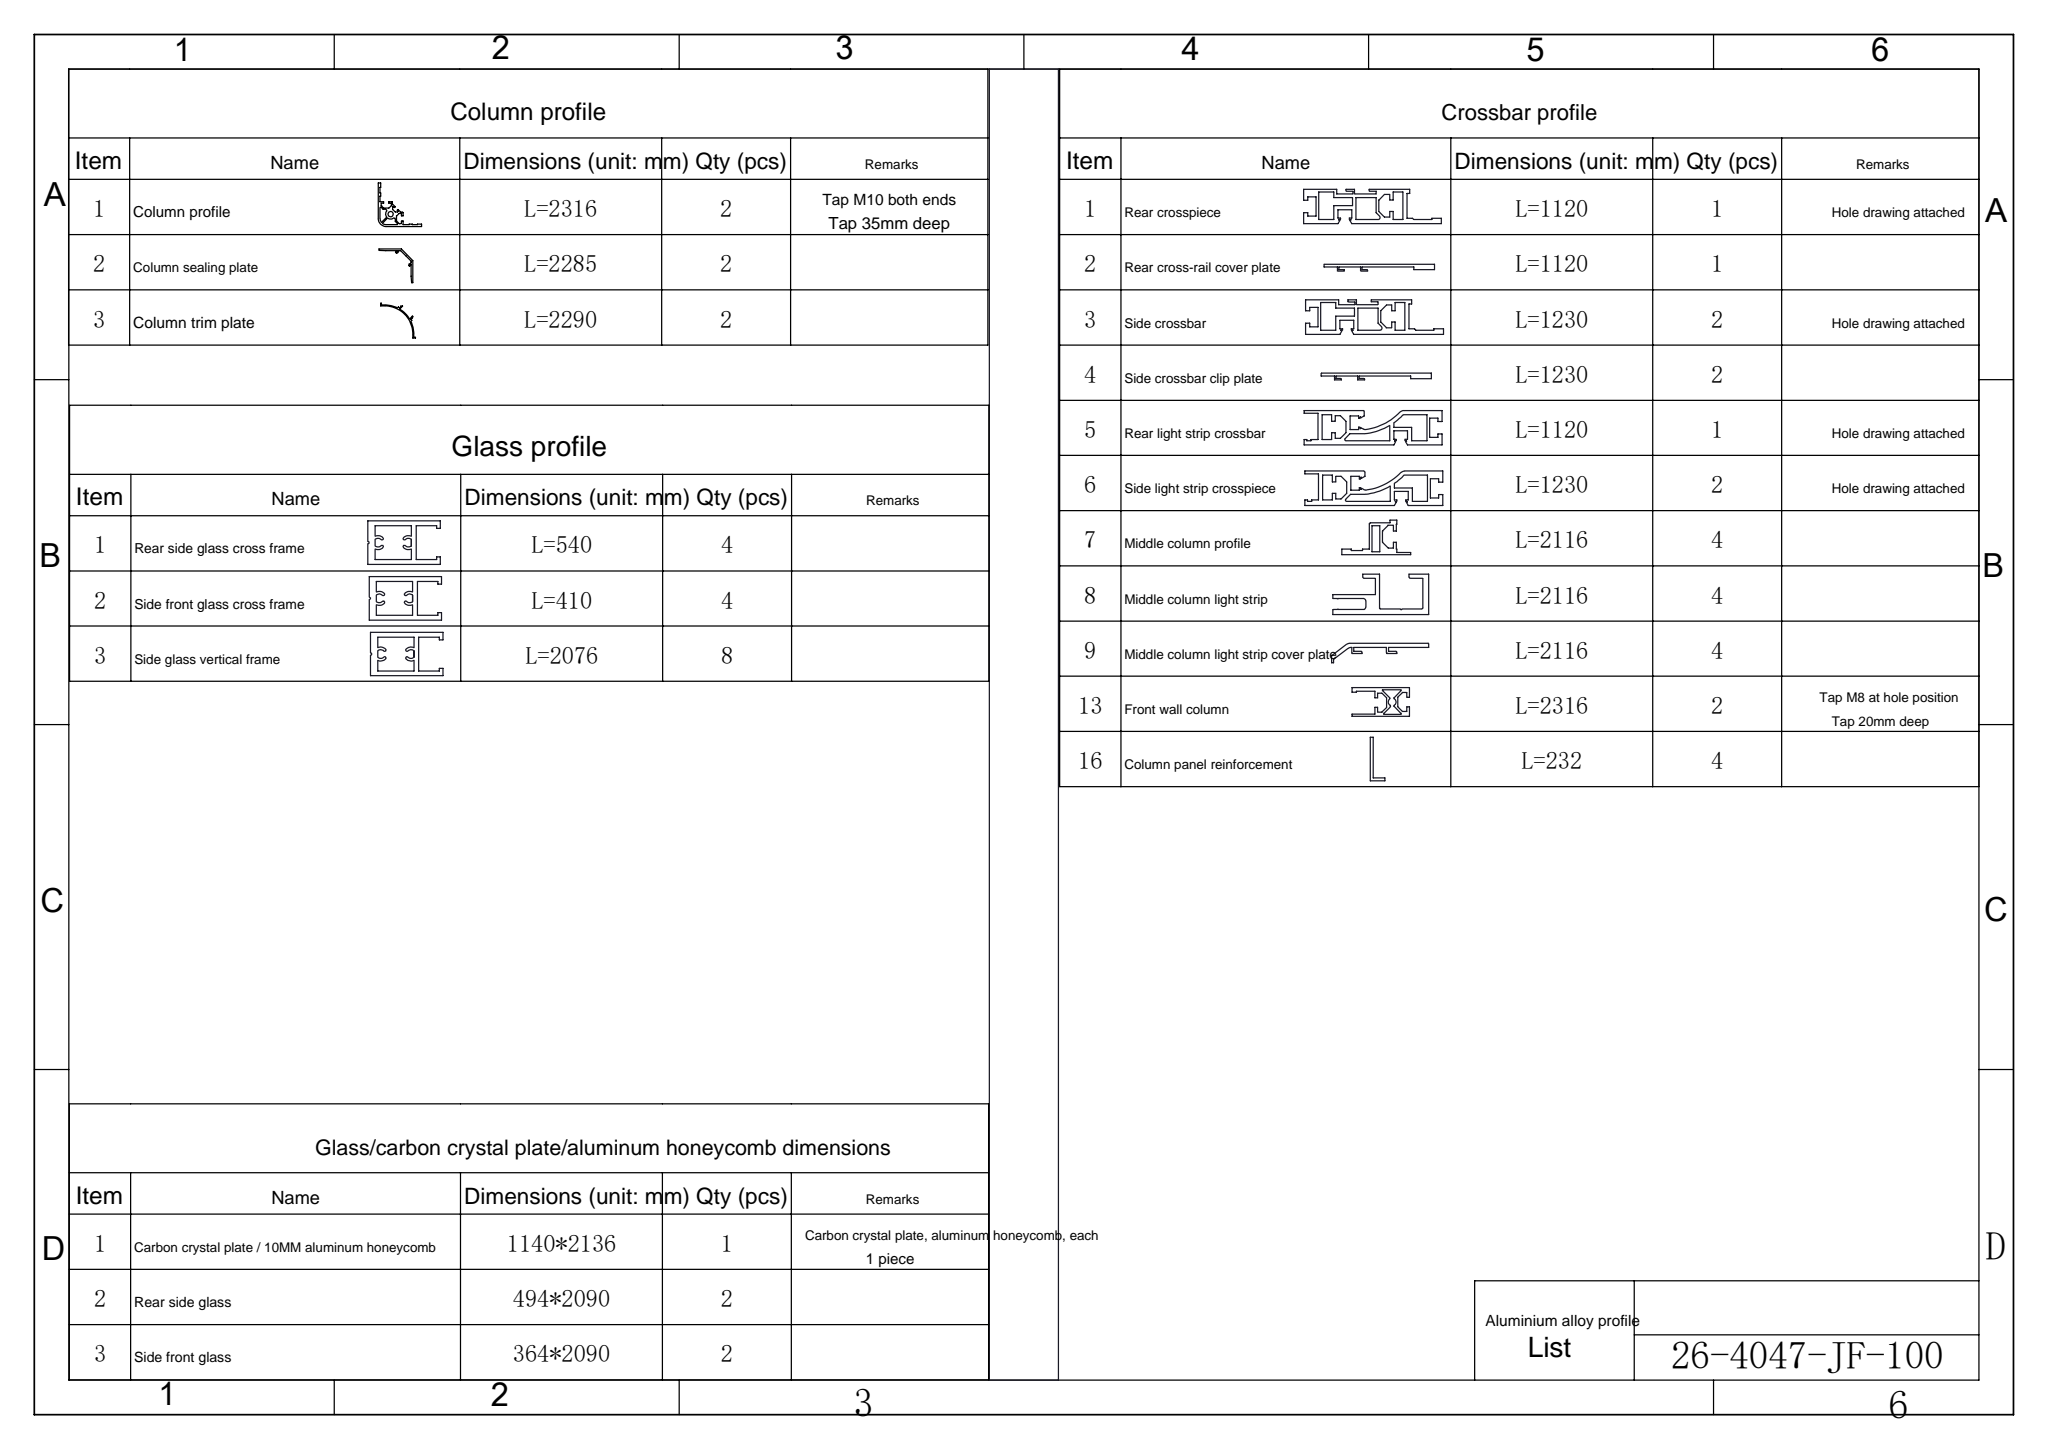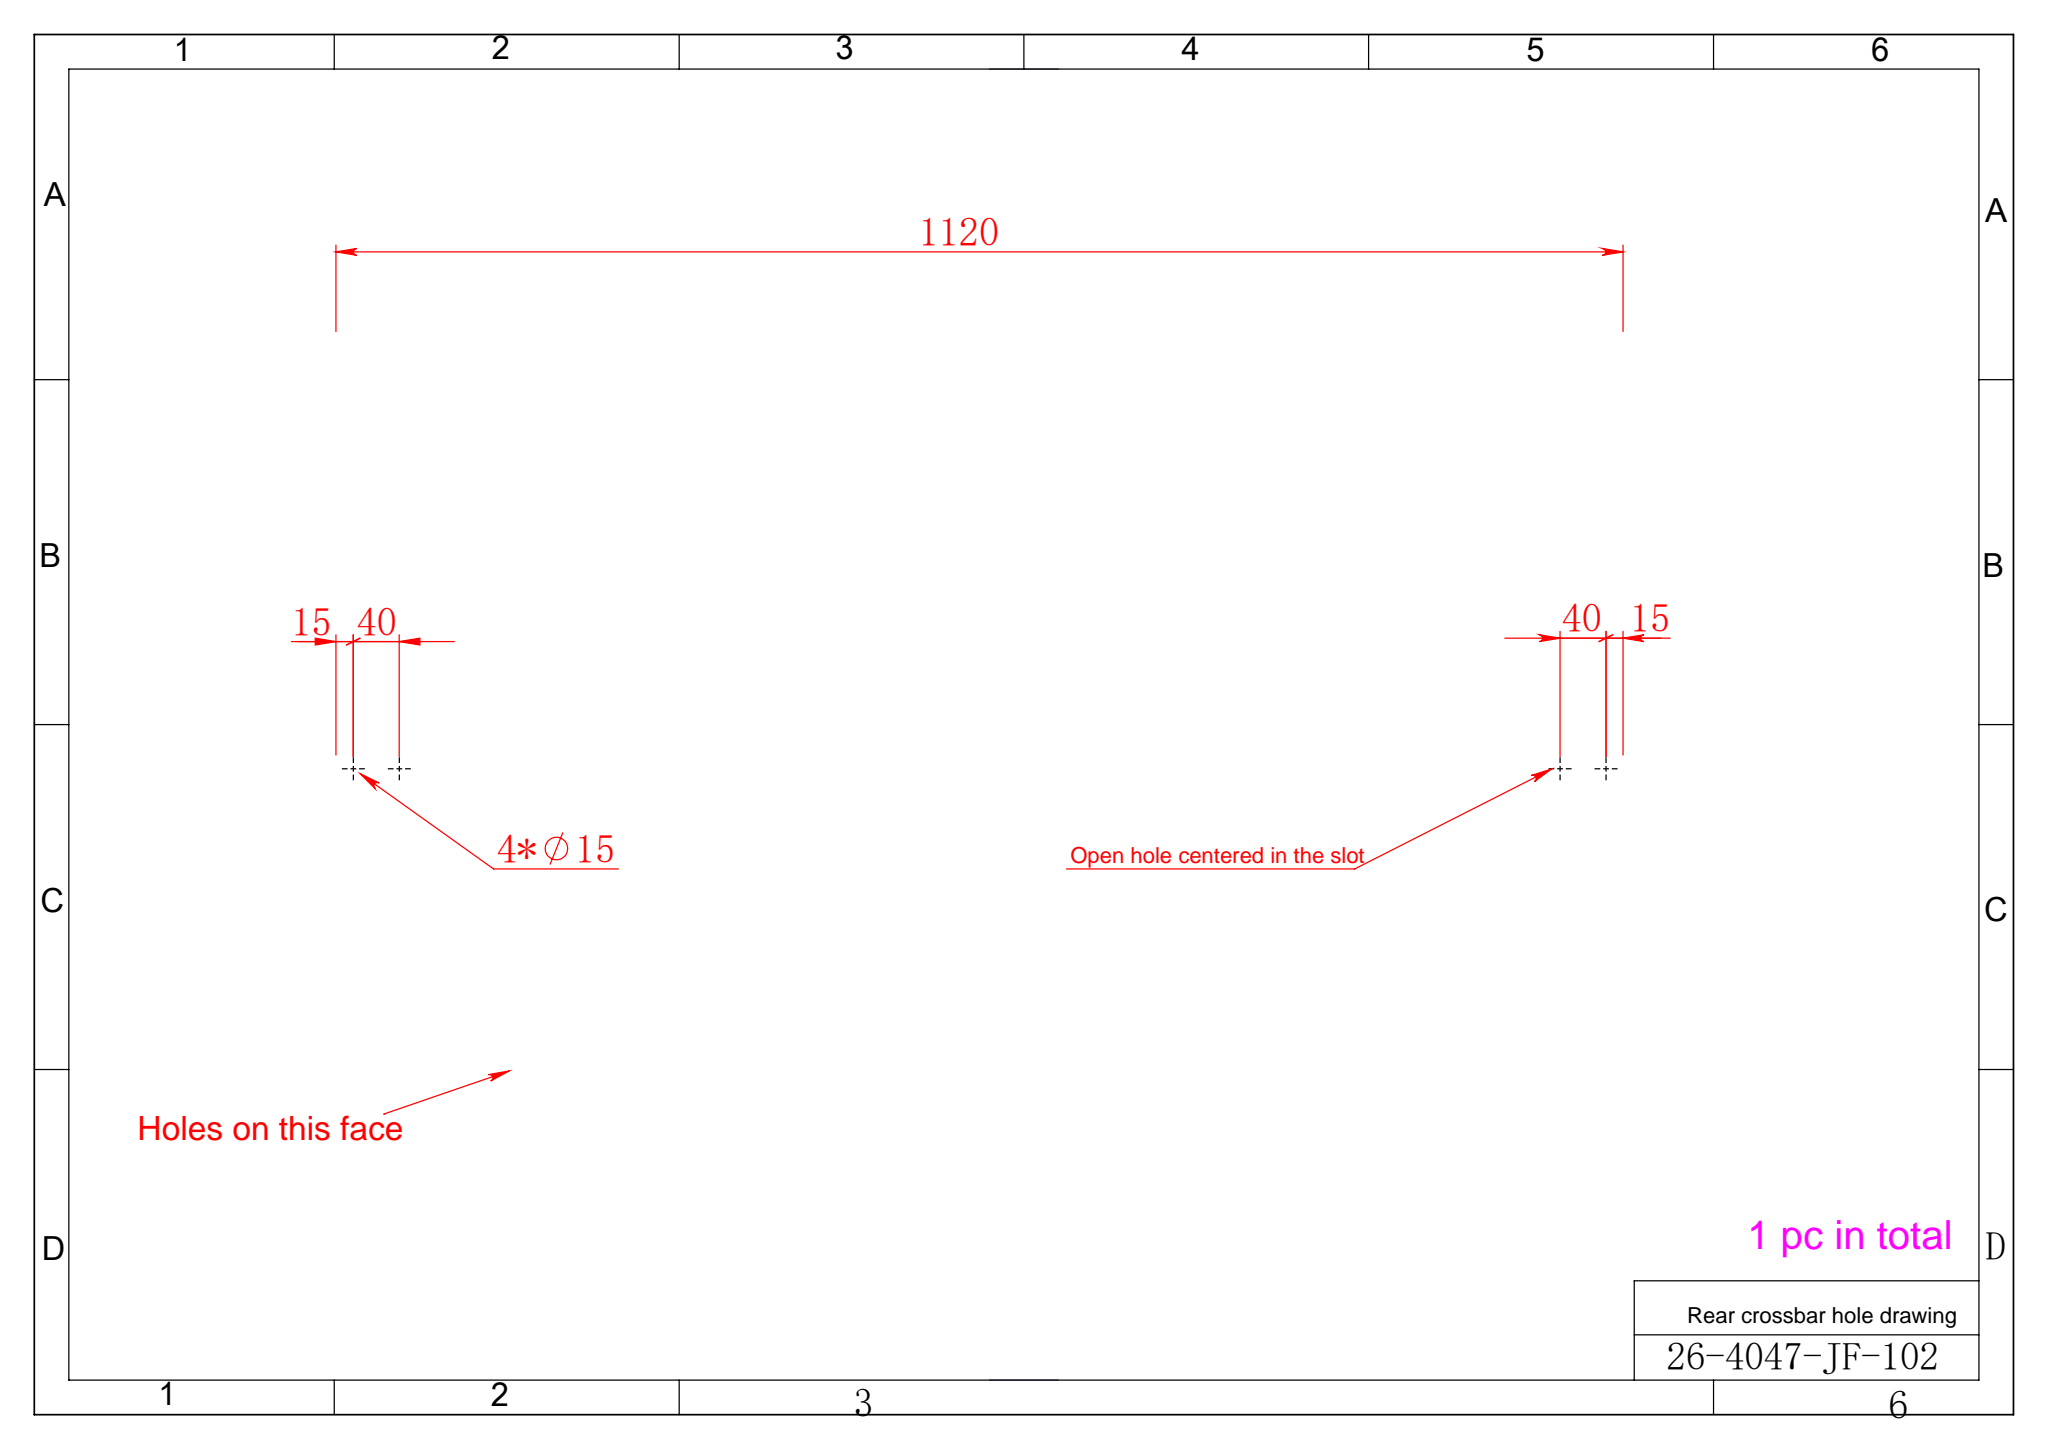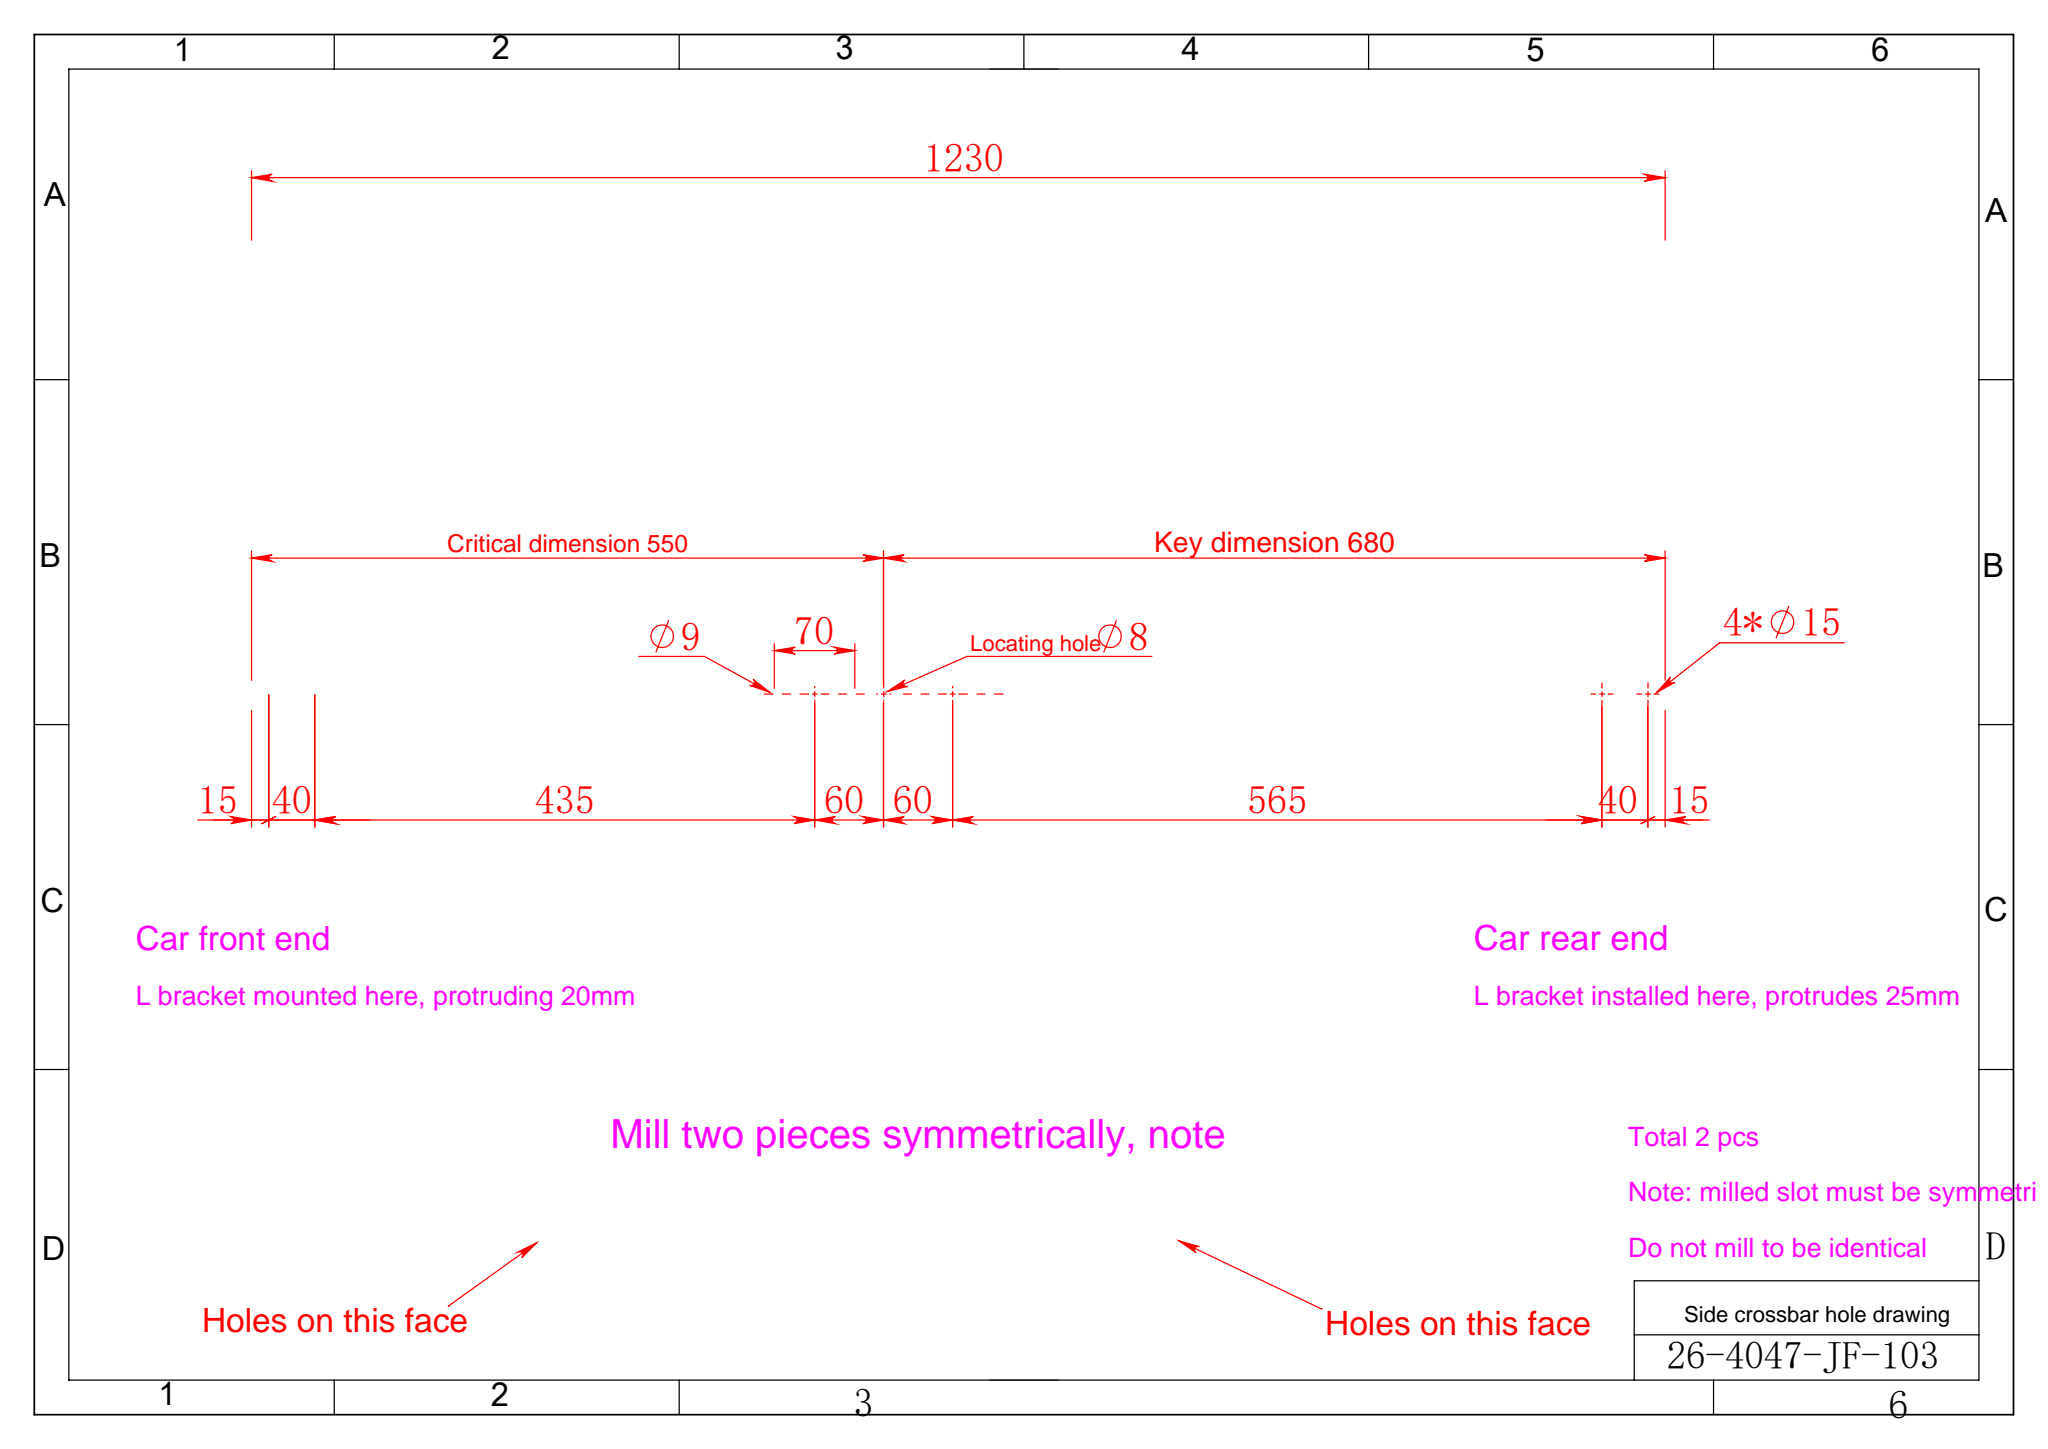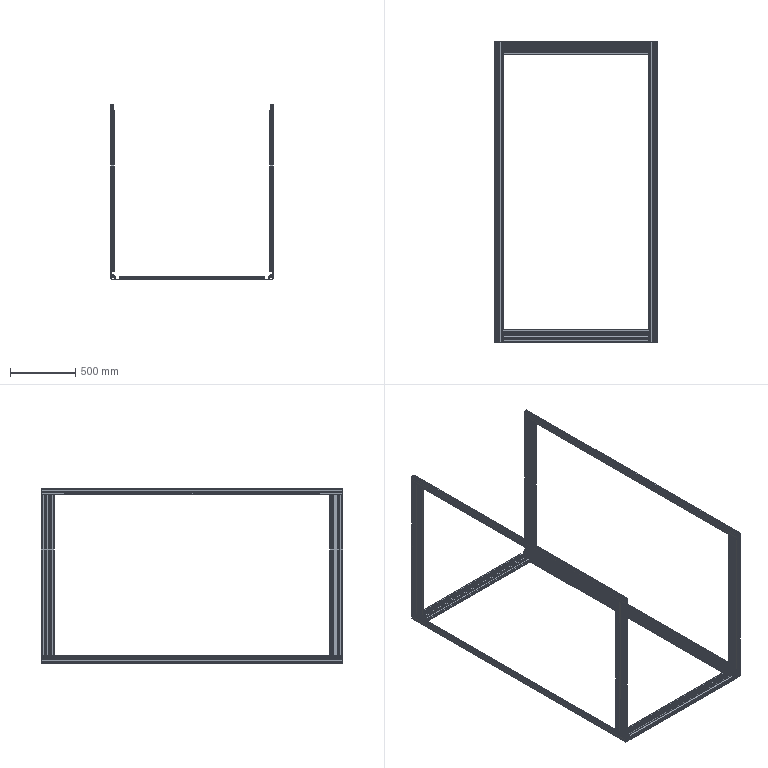Part | SolidWorks | features WeldMemberFeat 5, ICE 4, 3DProfileFeature 1, WeldmentFeature 1 | 13 solids | 1103 faces | box 1250 x 2316 x 1345 mm | volume 13061809 mm3 | plane 770 | cylinder 333 | commonest cylinder face diameters 0.6 x80 0.4 x63 15 x48 2 x24 0.24 x18 9 x18